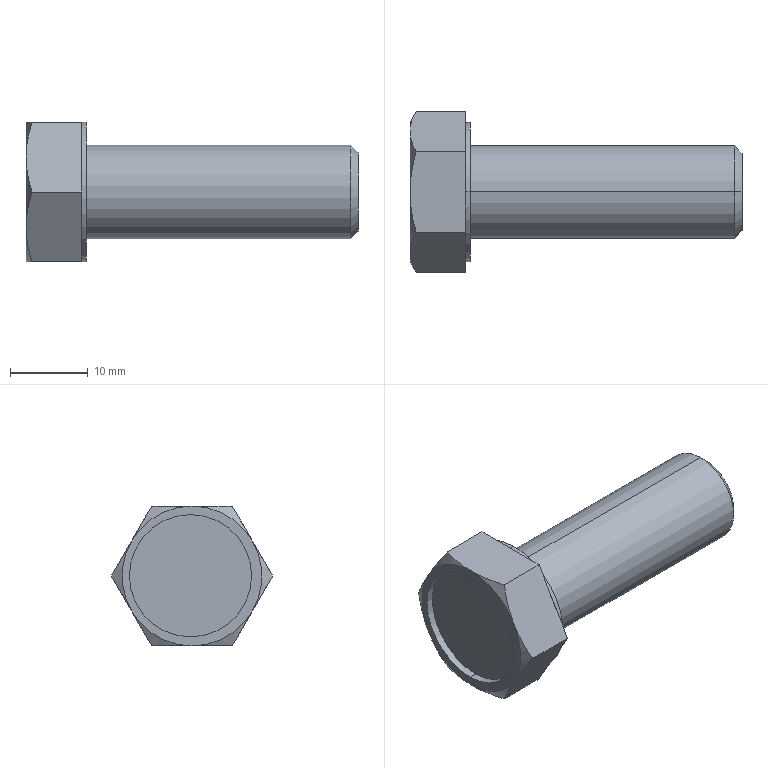Part | STEP file | formed hex screw_am_B18.2.3.2M - Formed hex screw, M12 x 1.75 x 35 --35WN | 1 solid | 30 faces | box 42.76 x 20.785 x 18 mm | volume 5908 mm3 | plane 16 | cone 8 | cylinder 6 | commonest cylinder face diameters 12 x2 15.75 x2 18 x2